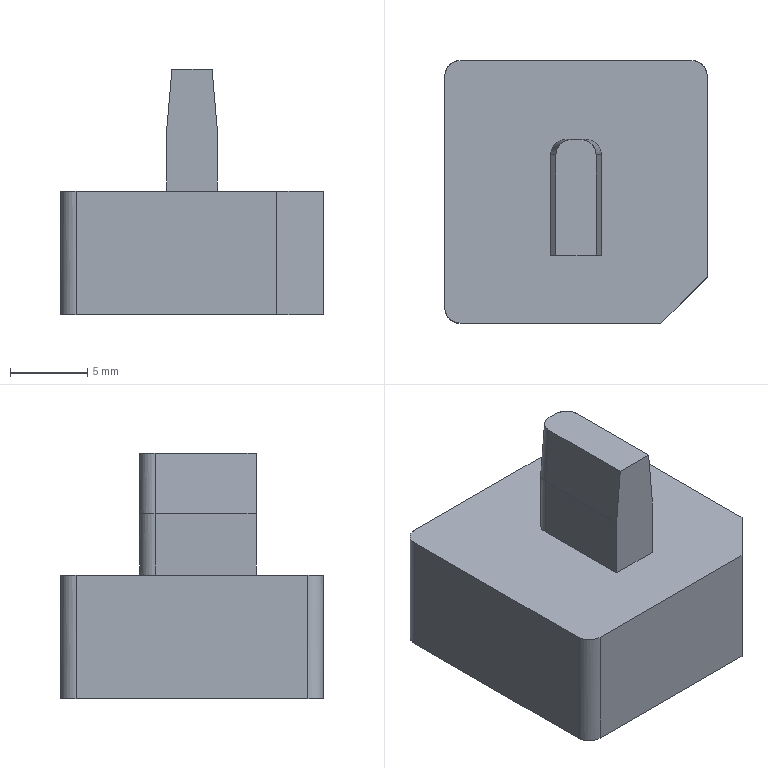NC program | PowerMill | posted with a generic post | part box 17 x 17 x 15.883 mm
Lines 1 to 1082 of 37483:
%
O0001
N104 ( POWERMILL CB  : 2026004.0)
N105 ( POST VER      : 2026.0.0.5161)
N106 ( OPTION FILE   : FANUC)
N107 ( OUTPUT WORKPLANE : WORLD)
N108 (  )
N109 ( TOOL LIST )
N110 (---------------------------------------)
N111 ( NO. | ID        | DIA.| TIP RAD|LENGTH)
N112 (---------------------------------------)
N113 (    1|D10C_1_1   |10.0 |  0.0   |71.32 )
N114 (    3|D10_1_1    |10.0 |  0.0   |71.04 )
N115 (   14|D4_1_1     | 4.0 |  0.0   |63.04 )
N116 (   13|TEXT_D4_1_1| 4.0 |  0.3   |63.16 )
N117 (---------------------------------------)
N118 (  )
N119 ( NUMBER OF TOOLPATHS: 9.0 )
N120 ( ESTIMATED PROGRAM DURATION: 0 HOURS 4 MIN 27 SEC)
N121 (  )
N122 G00 G21 G80 G40 G17
N123 G90
N124 G54
N125 G53 Z0.0
N126 (---------------)
N127 ( START TOOLPATH : 精公开粗01-扫面平行-D10C )
N128 (---------------)
N129 ( TOOL NO.    :1 )
N130 ( TOOL TYPE   : ENDMILL)
N131 ( TOOL ID     : D10C_1_1)
N132 ( TOOL DIA    : 10.0 LENGTH 71.32)
N133 T1
N134 M6
N135 S8000 M03
N136 G00 G90 X0.0 Y0.0
N137 G43 Z10.2 H1
N138
N139 G05 P10000 R4
N140 X11.28 Y11.28
N141 Z1.134
N142 G01 Z-0.066 F6000.0
N143 X-11.28 F10000.0
N144 Y5.64
N145 X11.28
N146 Y0.0
N147 X-11.28
N148 Y-5.64
N149 X11.28
N150 Y-11.28
N151 X-11.28
N152 X-16.28
N153 G00 Z10.2
N154 G05 P0
N155 (---------------)
N156 ( END TOOLPATH : 精公开粗01-扫面平行-D10C )
N157 (---------------)
N158 ( START TOOLPATH : 精公开粗01-外形偏置-D10C )
N159 (---------------)
N160 G00 X0.0 Y-0.3245 Z9.884
N161 G05 P10000 R4
N162 X6.2233 Y-17.204
N163 Z0.6953
N164 G01 Z-0.5047 F6000.0
N165 Y-16.6765 F10000.0
N166 G03 X1.4758 Y-11.929 I-4.7475 J0.0
N167 G01 X-10.28
N168 G02 X-11.28 Y-10.929 I0.0 J1.0
N169 G01 Y10.28
N170 G02 X-10.28 Y11.28 I1.0 J0.0
N171 G01 X10.28
N172 G02 X11.28 Y10.28 I0.0 J-1.0
N173 G01 Y-10.929
N174 G02 X10.28 Y-11.929 I-1.0 J0.0
N175 G01 X1.4758
N176 X1.3535 Y-9.4205
N177 X1.1601 Y-9.4299
N178 X-1.1601
N179 X-1.9336 Y-9.3922
N180 X-2.707 Y-9.2455
N181 X-3.4804 Y-8.9698
N182 X-3.7658 Y-8.8322
N183 X-4.2538 Y-8.5428
N184 X-4.8751 Y-8.0588
N185 X-5.0273 Y-7.9148
N186 X-5.5738 Y-7.2853
N187 X-5.8007 Y-6.9515
N188 X-6.0478 Y-6.5119
N189 X-6.3609 Y-5.7385
N190 X-6.5423 Y-4.9651
N191 X-6.6054 Y-4.1916
N192 X-6.6056 Y1.9958
N193 X-6.5917 Y2.7692
N194 X-6.4881 Y3.5426
N195 X-6.3018 Y4.3161
N196 X-5.9828 Y5.0895
N197 X-5.554 Y5.8629
N198 X-5.0273 Y6.5406
N199 X-4.2538 Y7.2833
N200 X-3.4804 Y7.8088
N201 X-2.7303 Y8.1832
N202 X-1.9336 Y8.455
N203 X-1.1601 Y8.6004
N204 X-0.3867 Y8.6667
N205 X0.3867
N206 X1.1601 Y8.6064
N207 X1.9336 Y8.4558
N208 X2.7363 Y8.1832
N209 X3.4804 Y7.8114
N210 X4.2538 Y7.285
N211 X4.9451 Y6.6363
N212 X5.5496 Y5.8629
N213 X5.8007 Y5.4567
N214 X5.994 Y5.0895
N215 X6.297 Y4.3161
N216 X6.4973 Y3.5426
N217 X6.5741 Y2.9617
N218 X6.6056 Y1.9958
N219 X6.6054 Y-4.1916
N220 X6.5423 Y-4.9651
N221 X6.3609 Y-5.7385
N222 X6.0478 Y-6.5119
N223 X5.8007 Y-6.9515
N224 X5.5738 Y-7.2853
N225 X5.0273 Y-7.9148
N226 X4.8751 Y-8.0588
N227 X4.2538 Y-8.5428
N228 X3.7658 Y-8.8322
N229 X3.4804 Y-8.9698
N230 X2.707 Y-9.2455
N231 X1.9336 Y-9.3922
N232 X1.3535 Y-9.4205
N233 X1.4758 Y-11.929
N234 G00 Z3.3066
N235 G01 X6.2233 Y-17.204
N236 G00 Z0.3066
N237 G01 Z-0.8934 F6000.0
N238 Y-16.6765 F10000.0
N239 G03 X1.4758 Y-11.929 I-4.7475 J0.0
N240 G01 X1.3581
N241 X1.2568 Y-9.426
N242 X1.1601 Y-9.4299
N243 X-1.1601
N244 X-1.9336 Y-9.3986
N245 X-2.707 Y-9.254
N246 X-3.4804 Y-8.9845
N247 X-3.7998 Y-8.8322
N248 X-4.2538 Y-8.5647
N249 X-4.9091 Y-8.0588
N250 X-5.6078 Y-7.2853
N251 X-5.8007 Y-7.0056
N252 X-6.0818 Y-6.5119
N253 X-6.395 Y-5.7385
N254 X-6.5741 Y-4.9786
N255 X-6.6394 Y-4.1916
N256 X-6.6396 Y1.9958
N257 X-6.6257 Y2.7692
N258 X-6.5221 Y3.5426
N259 X-6.3358 Y4.3161
N260 X-6.0168 Y5.0895
N261 X-5.588 Y5.8629
N262 X-5.0273 Y6.5771
N263 X-4.2538 Y7.3101
N264 X-3.4804 Y7.8271
N265 X-2.7643 Y8.1832
N266 X-1.9336 Y8.4632
N267 X-1.1601 Y8.6054
N268 X-0.3867 Y8.667
N269 X0.3867
N270 X1.1601 Y8.6109
N271 X1.9336 Y8.4645
N272 X2.707 Y8.208
N273 X3.4804 Y7.8315
N274 X4.1268 Y7.4098
N275 X4.9794 Y6.6363
N276 X5.5835 Y5.8629
N277 X6.028 Y5.0895
N278 X6.3309 Y4.3161
N279 X6.5314 Y3.5426
N280 X6.6257 Y2.7692
N281 X6.6396 Y1.9958
N282 X6.6394 Y-4.1916
N283 X6.5763 Y-4.9651
N284 X6.395 Y-5.7385
N285 X6.0818 Y-6.5119
N286 X5.8007 Y-7.0056
N287 X5.6078 Y-7.2853
N288 X5.0273 Y-7.947
N289 X4.2538 Y-8.5647
N290 X3.7998 Y-8.8322
N291 X3.4804 Y-8.9845
N292 X2.707 Y-9.254
N293 X1.9336 Y-9.3986
N294 X1.2568 Y-9.426
N295 X1.3581 Y-11.929
N296 X-10.28
N297 G02 X-11.28 Y-10.929 I0.0 J1.0
N298 G01 Y10.28
N299 G02 X-10.28 Y11.28 I1.0 J0.0
N300 G01 X10.28
N301 G02 X11.28 Y10.28 I0.0 J-1.0
N302 G01 Y-10.929
N303 G02 X10.28 Y-11.929 I-1.0 J0.0
N304 G01 X1.4758
N305 G00 Z2.9179
N306 G01 X6.2233 Y-17.204
N307 G00 Z-0.0821
N308 G01 Z-1.2821 F6000.0
N309 Y-16.6765 F10000.0
N310 G03 X1.4758 Y-11.929 I-4.7475 J0.0
N311 G01 X1.1601
N312 Y-9.4299
N313 X-1.1601
N314 X-1.9336 Y-9.4022
N315 X-2.707 Y-9.2626
N316 X-3.4804 Y-8.9992
N317 X-3.8338 Y-8.8322
N318 X-4.2538 Y-8.5867
N319 X-4.9431 Y-8.0588
N320 X-5.6418 Y-7.2853
N321 X-5.8007 Y-7.057
N322 X-6.1158 Y-6.5119
N323 X-6.429 Y-5.7385
N324 X-6.6103 Y-4.9651
N325 X-6.6734 Y-4.1916
N326 X-6.6736 Y1.9958
N327 X-6.6597 Y2.7692
N328 X-6.5741 Y3.4297
N329 X-6.3698 Y4.3161
N330 X-6.0508 Y5.0895
N331 X-5.622 Y5.8629
N332 X-5.0273 Y6.6135
N333 X-4.2538 Y7.3369
N334 X-3.4804 Y7.8453
N335 X-2.7983 Y8.1832
N336 X-1.9336 Y8.4715
N337 X-1.1601 Y8.6104
N338 X-0.3867 Y8.667
N339 X0.3867
N340 X1.1601 Y8.6153
N341 X1.9336 Y8.4729
N342 X2.707 Y8.2211
N343 X3.4804 Y7.8515
N344 X4.1607 Y7.4098
N345 X5.0138 Y6.6363
N346 X5.6174 Y5.8629
N347 X6.062 Y5.0895
N348 X6.3648 Y4.3161
N349 X6.5654 Y3.5426
N350 X6.6597 Y2.7692
N351 X6.6735 Y1.9958
N352 X6.6734 Y-4.1916
N353 X6.6103 Y-4.9651
N354 X6.429 Y-5.7385
N355 X6.1158 Y-6.5119
N356 X5.8007 Y-7.057
N357 X5.6418 Y-7.2853
N358 X5.0273 Y-7.9791
N359 X4.2538 Y-8.5867
N360 X3.8338 Y-8.8322
N361 X3.4804 Y-8.9992
N362 X2.707 Y-9.2626
N363 X1.9336 Y-9.4022
N364 X1.1601 Y-9.4299
N365 Y-11.929
N366 X-10.28
N367 G02 X-11.28 Y-10.929 I0.0 J1.0
N368 G01 Y10.28
N369 G02 X-10.28 Y11.28 I1.0 J0.0
N370 G01 X10.28
N371 G02 X11.28 Y10.28 I0.0 J-1.0
N372 G01 Y-10.929
N373 G02 X10.28 Y-11.929 I-1.0 J0.0
N374 G01 X1.4758
N375 G00 Z2.5292
N376 G01 X6.2233 Y-17.204
N377 G00 Z-0.4708
N378 G01 Z-1.6708 F6000.0
N379 Y-16.6765 F10000.0
N380 G03 X1.4758 Y-11.929 I-4.7475 J0.0
N381 G01 X1.1601
N382 Y-9.4299
N383 X-1.1601
N384 X-1.9336 Y-9.4056
N385 X-2.707 Y-9.2711
N386 X-3.4804 Y-9.0138
N387 X-3.8678 Y-8.8322
N388 X-4.2538 Y-8.6086
N389 X-4.9771 Y-8.0588
N390 X-5.6758 Y-7.2853
N391 X-6.1497 Y-6.5119
N392 X-6.463 Y-5.7385
N393 X-6.6443 Y-4.9651
N394 X-6.7074 Y-4.1916
N395 X-6.7076 Y1.9958
N396 X-6.6937 Y2.7692
N397 X-6.5902 Y3.5426
N398 X-6.4038 Y4.3161
N399 X-6.0848 Y5.0895
N400 X-5.656 Y5.8629
N401 X-5.04 Y6.6363
N402 X-4.2538 Y7.3637
N403 X-3.4804 Y7.8636
N404 X-2.8323 Y8.1832
N405 X-1.9336 Y8.4798
N406 X-1.1601 Y8.6154
N407 X-0.3867 Y8.667
N408 X0.3867
N409 X1.1601 Y8.6197
N410 X1.9336 Y8.4814
N411 X2.707 Y8.2343
N412 X3.4804 Y7.8715
N413 X4.1947 Y7.4098
N414 X5.048 Y6.6363
N415 X5.6513 Y5.8629
N416 X6.096 Y5.0895
N417 X6.3987 Y4.3161
N418 X6.5741 Y3.6729
N419 X6.6938 Y2.7692
N420 X6.7075 Y1.9958
N421 X6.7074 Y-4.1916
N422 X6.6443 Y-4.9651
N423 X6.463 Y-5.7385
N424 X6.1497 Y-6.5119
N425 X5.6758 Y-7.2853
N426 X5.0273 Y-8.0113
N427 X4.2538 Y-8.6086
N428 X3.8678 Y-8.8322
N429 X3.4804 Y-9.0138
N430 X2.707 Y-9.2711
N431 X1.9336 Y-9.4056
N432 X1.1601 Y-9.4299
N433 Y-11.929
N434 X-10.28
N435 G02 X-11.28 Y-10.929 I0.0 J1.0
N436 G01 Y10.28
N437 G02 X-10.28 Y11.28 I1.0 J0.0
N438 G01 X10.28
N439 G02 X11.28 Y10.28 I0.0 J-1.0
N440 G01 Y-10.929
N441 G02 X10.28 Y-11.929 I-1.0 J0.0
N442 G01 X1.4758
N443 G00 Z2.1405
N444 G01 X6.2233 Y-17.204
N445 G00 Z-0.8595
N446 G01 Z-2.0595 F6000.0
N447 Y-16.6765 F10000.0
N448 G03 X1.4758 Y-11.929 I-4.7475 J0.0
N449 G01 X-10.28
N450 G02 X-11.28 Y-10.929 I0.0 J1.0
N451 G01 Y10.28
N452 G02 X-10.28 Y11.28 I1.0 J0.0
N453 G01 X10.28
N454 G02 X11.28 Y10.28 I0.0 J-1.0
N455 G01 Y-10.929
N456 G02 X10.28 Y-11.929 I-1.0 J0.0
N457 G01 X2.0024
N458 X1.9336 Y-9.4088
N459 X1.1601 Y-9.4299
N460 X-1.1601
N461 X-1.9336 Y-9.4088
N462 X-2.707 Y-9.2796
N463 X-3.4804 Y-9.0285
N464 X-3.9018 Y-8.8322
N465 X-4.2538 Y-8.6306
N466 X-5.0111 Y-8.0588
N467 X-5.7098 Y-7.2853
N468 X-6.1837 Y-6.5119
N469 X-6.497 Y-5.7385
N470 X-6.6783 Y-4.9651
N471 X-6.7413 Y-4.1916
N472 X-6.7416 Y1.9958
N473 X-6.7277 Y2.7692
N474 X-6.6242 Y3.5426
N475 X-6.4378 Y4.3161
N476 X-6.1188 Y5.0895
N477 X-5.69 Y5.8629
N478 X-5.074 Y6.6363
N479 X-4.2294 Y7.4098
N480 X-3.4804 Y7.8819
N481 X-2.8663 Y8.1832
N482 X-1.9336 Y8.4878
N483 X-1.1601 Y8.6201
N484 X-0.3867 Y8.667
N485 X0.3867
N486 X1.1601 Y8.624
N487 X1.9336 Y8.4899
N488 X2.707 Y8.2474
N489 X3.4804 Y7.8914
N490 X4.2286 Y7.4098
N491 X5.0273 Y6.694
N492 X5.6852 Y5.8629
N493 X6.13 Y5.0895
N494 X6.4326 Y4.3161
N495 X6.6336 Y3.5426
N496 X6.7278 Y2.7692
N497 X6.7415 Y1.9958
N498 X6.7414 Y-4.1916
N499 X6.6783 Y-4.9651
N500 X6.497 Y-5.7385
N501 X6.1837 Y-6.5119
N502 X5.7098 Y-7.2853
N503 X5.0111 Y-8.0588
N504 X4.2538 Y-8.6306
N505 X3.9018 Y-8.8322
N506 X3.4804 Y-9.0285
N507 X2.707 Y-9.2796
N508 X1.9336 Y-9.4088
N509 X2.0024 Y-11.929
N510 X1.4758
N511 G00 Z1.7518
N512 G01 X6.2233 Y-17.204
N513 G00 Z-1.2482
N514 G01 Z-2.4482 F6000.0
N515 Y-16.6765 F10000.0
N516 G03 X1.4758 Y-11.929 I-4.7475 J0.0
N517 G01 X-10.28
N518 G02 X-11.28 Y-10.929 I0.0 J1.0
N519 G01 Y10.28
N520 G02 X-10.28 Y11.28 I1.0 J0.0
N521 G01 X10.28
N522 G02 X11.28 Y10.28 I0.0 J-1.0
N523 G01 Y-10.929
N524 G02 X10.28 Y-11.929 I-1.0 J0.0
N525 G01 X1.9931
N526 X1.9336 Y-9.4117
N527 X1.1601 Y-9.4299
N528 X1.1509
N529 X-1.1601
N530 X-1.7978 Y-9.4125
N531 X-1.9336 Y-9.4117
N532 X-2.707 Y-9.2881
N533 X-3.4804 Y-9.0423
N534 X-3.9358 Y-8.8322
N535 X-4.2538 Y-8.652
N536 X-5.0451 Y-8.0588
N537 X-5.7439 Y-7.2853
N538 X-6.2177 Y-6.5119
N539 X-6.531 Y-5.7385
N540 X-6.7123 Y-4.9651
N541 X-6.7753 Y-4.1916
N542 X-6.7756 Y1.9958
N543 X-6.7617 Y2.7692
N544 X-6.6582 Y3.5426
N545 X-6.4718 Y4.3161
N546 X-6.1528 Y5.0895
N547 X-5.8007 Y5.7413
N548 X-5.108 Y6.6363
N549 X-4.2634 Y7.4098
N550 X-3.4804 Y7.8997
N551 X-2.707 Y8.2616
N552 X-1.9336 Y8.4954
N553 X-1.1601 Y8.6245
N554 X-0.3867 Y8.667
N555 X0.3867
N556 X1.1601 Y8.6282
N557 X1.9336 Y8.4983
N558 X2.707 Y8.2605
N559 X3.4804 Y7.9096
N560 X4.2538 Y7.4162
N561 X5.0273 Y6.7299
N562 X5.7191 Y5.8629
N563 X6.164 Y5.0895
N564 X6.4665 Y4.3161
N565 X6.5741 Y3.9618
N566 X6.6677 Y3.5426
N567 X6.7618 Y2.7692
N568 X6.7755 Y1.9958
N569 X6.7754 Y-4.1916
N570 X6.7123 Y-4.9651
N571 X6.5741 Y-5.5936
N572 X6.2177 Y-6.5119
N573 X5.8007 Y-7.2051
N574 X5.0451 Y-8.0588
N575 X4.2538 Y-8.652
N576 X3.9358 Y-8.8322
N577 X3.4804 Y-9.0423
N578 X2.707 Y-9.2881
N579 X1.9336 Y-9.4117
N580 X1.9931 Y-11.929
N581 X1.4758
N582 G00 Z1.3631
N583 G01 X6.2233 Y-17.204
N584 G00 Z-1.6369
N585 G01 Z-2.8369 F6000.0
N586 Y-16.6765 F10000.0
N587 G03 X1.4758 Y-11.929 I-4.7475 J0.0
N588 G01 X-10.28
N589 G02 X-11.28 Y-10.929 I0.0 J1.0
N590 G01 Y10.28
N591 G02 X-10.28 Y11.28 I1.0 J0.0
N592 G01 X10.28
N593 G02 X11.28 Y10.28 I0.0 J-1.0
N594 G01 Y-10.929
N595 G02 X10.28 Y-11.929 I-1.0 J0.0
N596 G01 X1.984
N597 X1.9336 Y-9.4144
N598 X1.1601 Y-9.4299
N599 X1.1383 Y-9.4298
N600 X-1.1601
N601 X-1.677 Y-9.4157
N602 X-1.9336 Y-9.4144
N603 X-2.707 Y-9.2966
N604 X-3.4804 Y-9.0556
N605 X-3.9698 Y-8.8322
N606 X-4.2538 Y-8.6721
N607 X-5.0273 Y-8.104
N608 X-5.7779 Y-7.2853
N609 X-6.2517 Y-6.5119
N610 X-6.565 Y-5.7385
N611 X-6.7463 Y-4.9651
N612 X-6.8093 Y-4.1916
N613 X-6.8096 Y1.9958
N614 X-6.7957 Y2.7692
N615 X-6.6922 Y3.5426
N616 X-6.5058 Y4.3161
N617 X-6.1868 Y5.0895
N618 X-5.8007 Y5.796
N619 X-5.142 Y6.6363
N620 X-4.2974 Y7.4098
N621 X-3.4804 Y7.9171
N622 X-2.707 Y8.2754
N623 X-1.9336 Y8.5027
N624 X-1.1601 Y8.6288
N625 X-0.3867 Y8.667
N626 X0.3867
N627 X1.1601 Y8.6323
N628 X1.9336 Y8.5068
N629 X2.707 Y8.2736
N630 X3.4804 Y7.9278
N631 X4.2538 Y7.441
N632 X5.1506 Y6.6363
N633 X5.753 Y5.8629
N634 X6.198 Y5.0895
N635 X6.5003 Y4.3161
N636 X6.7018 Y3.5426
N637 X6.7958 Y2.7692
N638 X6.8095 Y1.9958
N639 X6.8094 Y-4.1916
N640 X6.7463 Y-4.9651
N641 X6.565 Y-5.7385
N642 X6.2517 Y-6.5119
N643 X5.8007 Y-7.2531
N644 X5.0791 Y-8.0588
N645 X4.2538 Y-8.6721
N646 X3.9698 Y-8.8322
N647 X3.4804 Y-9.0556
N648 X2.707 Y-9.2966
N649 X1.9336 Y-9.4144
N650 X1.984 Y-11.929
N651 X1.4758
N652 G00 Z0.9744
N653 G01 X6.2233 Y-17.204
N654 G00 Z-2.0256
N655 G01 Z-3.2256 F6000.0
N656 Y-16.6765 F10000.0
N657 G03 X1.4758 Y-11.929 I-4.7475 J0.0
N658 G01 X-10.28
N659 G02 X-11.28 Y-10.929 I0.0 J1.0
N660 G01 Y10.28
N661 G02 X-10.28 Y11.28 I1.0 J0.0
N662 G01 X10.28
N663 G02 X11.28 Y10.28 I0.0 J-1.0
N664 G01 Y-10.929
N665 G02 X10.28 Y-11.929 I-1.0 J0.0
N666 G01 X1.9336
N667 Y-9.417
N668 X1.8047
N669 X1.1601 Y-9.4299
N670 X1.1383 Y-9.4298
N671 X-1.1601
N672 X-1.6295 Y-9.417
N673 X-1.9336
N674 X-2.707 Y-9.3046
N675 X-3.4804 Y-9.0689
N676 X-4.0038 Y-8.8322
N677 X-4.2538 Y-8.6923
N678 X-5.0273 Y-8.1336
N679 X-5.8007 Y-7.3
N680 X-6.2857 Y-6.5119
N681 X-6.5741 Y-5.8139
N682 X-6.7803 Y-4.9651
N683 X-6.8433 Y-4.1916
N684 X-6.8436 Y1.9958
N685 X-6.8297 Y2.7692
N686 X-6.7262 Y3.5426
N687 X-6.5741 Y4.2046
N688 X-6.2209 Y5.0895
N689 X-5.8007 Y5.8493
N690 X-5.176 Y6.6363
N691 X-4.3314 Y7.4098
N692 X-3.4804 Y7.9346
N693 X-2.707 Y8.2879
N694 X-1.9336 Y8.5098
N695 X-1.1601 Y8.6328
N696 X-0.3867 Y8.667
N697 X0.3867
N698 X1.1601 Y8.6364
N699 X1.9336 Y8.5146
N700 X2.707 Y8.2867
N701 X3.4804 Y7.946
N702 X4.2538 Y7.4659
N703 X5.0273 Y6.8016
N704 X5.1848 Y6.6363
N705 X5.7868 Y5.8629
N706 X6.232 Y5.0895
N707 X6.5342 Y4.3161
N708 X6.7359 Y3.5426
N709 X6.8298 Y2.7692
N710 X6.8435 Y1.9958
N711 X6.8434 Y-4.1916
N712 X6.7803 Y-4.9651
N713 X6.599 Y-5.7385
N714 X6.2857 Y-6.5119
N715 X5.8119 Y-7.2853
N716 X5.1131 Y-8.0588
N717 X4.2538 Y-8.6923
N718 X4.0038 Y-8.8322
N719 X3.4804 Y-9.0689
N720 X2.707 Y-9.3046
N721 X1.9336 Y-9.417
N722 Y-11.929
N723 X1.4758
N724 G00 Z0.5857
N725 G01 X6.2233 Y-17.204
N726 G00 Z-2.4143
N727 G01 Z-3.6143 F6000.0
N728 Y-16.6765 F10000.0
N729 G03 X1.4758 Y-11.929 I-4.7475 J0.0
N730 G01 X-10.28
N731 G02 X-11.28 Y-10.929 I0.0 J1.0
N732 G01 Y10.28
N733 G02 X-10.28 Y11.28 I1.0 J0.0
N734 G01 X10.28
N735 G02 X11.28 Y10.28 I0.0 J-1.0
N736 G01 Y-10.929
N737 G02 X10.28 Y-11.929 I-1.0 J0.0
N738 G01 X1.9336
N739 Y-9.4192
N740 X1.6884
N741 X1.1601 Y-9.4298
N742 X1.1383 Y-9.4297
N743 X-1.1601
N744 X-1.5441 Y-9.4192
N745 X-1.9336
N746 X-2.707 Y-9.3121
N747 X-3.4804 Y-9.0822
N748 X-3.9979 Y-8.8348
N749 X-4.0038 Y-8.8321
N750 X-4.0057 Y-8.8311
N751 X-4.2538 Y-8.7124
N752 X-5.1471 Y-8.0588
N753 X-5.8007 Y-7.3448
N754 X-6.3197 Y-6.5119
N755 X-6.5741 Y-5.914
N756 X-6.8143 Y-4.9651
N757 X-6.8773 Y-4.1916
N758 X-6.8776 Y1.9958
N759 X-6.8637 Y2.7692
N760 X-6.7602 Y3.5426
N761 X-6.5741 Y4.3151
N762 X-6.2549 Y5.0895
N763 X-5.8265 Y5.8629
N764 X-5.2101 Y6.6363
N765 X-4.3654 Y7.4098
N766 X-3.4804 Y7.952
N767 X-2.707 Y8.3004
N768 X-1.9336 Y8.5167
N769 X-1.1601 Y8.6365
N770 X-0.3867 Y8.6671
N771 X-0.3835 Y8.667
N772 X0.3867
N773 X0.9799 Y8.6435
N774 X1.1601 Y8.6404
N775 X1.9336 Y8.5222
N776 X2.707 Y8.2999
N777 X3.4804 Y7.9642
N778 X4.2538 Y7.4908
N779 X5.0273 Y6.8361
N780 X5.219 Y6.6363
N781 X5.8007 Y5.8936
N782 X6.266 Y5.0895
N783 X6.5681 Y4.3161
N784 X6.7699 Y3.5426
N785 X6.8638 Y2.7692
N786 X6.8775 Y1.9958
N787 X6.8774 Y-4.1916
N788 X6.8143 Y-4.9651
N789 X6.6329 Y-5.7385
N790 X6.3197 Y-6.5119
N791 X5.8458 Y-7.2853
N792 X5.1471 Y-8.0588
N793 X4.2538 Y-8.7124
N794 X4.0378 Y-8.8322
N795 X3.4804 Y-9.0822
N796 X2.707 Y-9.3121
N797 X1.9336 Y-9.4192
N798 Y-11.929
N799 X1.4758
N800 G00 Z0.197
N801 G01 X6.2233 Y-17.204
N802 G00 Z-2.803
N803 G01 Z-4.003 F6000.0
N804 Y-16.6765 F10000.0
N805 G03 X1.4758 Y-11.929 I-4.7475 J0.0
N806 G01 X-10.28
N807 G02 X-11.28 Y-10.929 I0.0 J1.0
N808 G01 Y10.28
N809 G02 X-10.28 Y11.28 I1.0 J0.0
N810 G01 X10.28
N811 G02 X11.28 Y10.28 I0.0 J-1.0
N812 G01 Y-10.929
N813 G02 X10.28 Y-11.929 I-1.0 J0.0
N814 G01 X1.9336
N815 Y-9.4213
N816 X1.5821
N817 X1.1601 Y-9.4298
N818 X1.1383 Y-9.4297
N819 X-1.1601
N820 X-1.466 Y-9.4213
N821 X-1.9336
N822 X-2.707 Y-9.3193
N823 X-3.4804 Y-9.0955
N824 X-4.2538 Y-8.7326
N825 X-5.0273 Y-8.1929
N826 X-5.1811 Y-8.0588
N827 X-5.8007 Y-7.3896
N828 X-6.3537 Y-6.5119
N829 X-6.6669 Y-5.7385
N830 X-6.8483 Y-4.9651
N831 X-6.9113 Y-4.1916
N832 X-6.9116 Y1.9958
N833 X-6.8977 Y2.7692
N834 X-6.7942 Y3.5426
N835 X-6.6078 Y4.3161
N836 X-6.2889 Y5.0895
N837 X-5.8611 Y5.8629
N838 X-5.2441 Y6.6363
N839 X-5.0273 Y6.8593
N840 X-4.3993 Y7.4098
N841 X-3.4804 Y7.9694
N842 X-3.0364 Y8.1832
N843 X-2.707 Y8.3128
N844 X-1.9336 Y8.5234
N845 X-1.1601 Y8.6401
N846 X-0.3867 Y8.6671
N847 X-0.3792 Y8.6669
N848 X0.3867
N849 X0.8394 Y8.649
N850 X1.1601 Y8.6443
N851 X1.9336 Y8.5297
N852 X2.707 Y8.313
N853 X3.4804 Y7.9824
N854 X4.2538 Y7.5157
N855 X5.0273 Y6.8707
N856 X5.2532 Y6.6363
N857 X5.8007 Y5.9454
N858 X6.3 Y5.0895
N859 X6.5741 Y4.3984
N860 X6.804 Y3.5426
N861 X6.8978 Y2.7692
N862 X6.9114 Y1.9958
N863 Y-4.1916
N864 X6.8483 Y-4.9651
N865 X6.6669 Y-5.7385
N866 X6.3537 Y-6.5119
N867 X5.8798 Y-7.2853
N868 X5.1811 Y-8.0588
N869 X5.0273 Y-8.1929
N870 X4.2538 Y-8.7326
N871 X4.0718 Y-8.8322
N872 X3.4804 Y-9.0955
N873 X2.707 Y-9.3193
N874 X1.9336 Y-9.4213
N875 Y-11.929
N876 X1.4758
N877 G00 Z-0.1917
N878 G01 X6.2233 Y-17.204
N879 G00 Z-3.1917
N880 G01 Z-4.3917 F6000.0
N881 Y-16.6765 F10000.0
N882 G03 X1.4758 Y-11.929 I-4.7475 J0.0
N883 G01 X-10.28
N884 G02 X-11.28 Y-10.929 I0.0 J1.0
N885 G01 Y10.28
N886 G02 X-10.28 Y11.28 I1.0 J0.0
N887 G01 X10.28
N888 G02 X11.28 Y10.28 I0.0 J-1.0
N889 G01 Y-10.929
N890 G02 X10.28 Y-11.929 I-1.0 J0.0
N891 G01 X1.9336
N892 Y-9.4218
N893 X1.557
N894 X1.1601 Y-9.4297
N895 X1.1383 Y-9.4296
N896 X-1.1601
N897 X-1.4476 Y-9.4218
N898 X-1.9336
N899 X-2.707 Y-9.3208
N900 X-3.4804 Y-9.0985
N901 X-4.2538 Y-8.737
N902 X-5.0273 Y-8.1995
N903 X-5.1887 Y-8.0588
N904 X-5.8007 Y-7.3994
N905 X-6.3613 Y-6.5119
N906 X-6.5741 Y-6.027
N907 X-6.6744 Y-5.7385
N908 X-6.8557 Y-4.9651
N909 X-6.9189 Y-4.1916
N910 X-6.919 Y1.9958
N911 X-6.9052 Y2.7692
N912 X-6.8116 Y3.5426
N913 X-6.6152 Y4.3161
N914 X-6.3059 Y5.0895
N915 X-5.8687 Y5.8629
N916 X-5.2606 Y6.6363
N917 X-5.0273 Y6.8783
N918 X-4.4069 Y7.4098
N919 X-3.4804 Y7.9826
N920 X-3.054 Y8.1832
N921 X-2.707 Y8.3156
N922 X-1.9336 Y8.5314
N923 X-1.1601 Y8.6409
N924 X-0.3867 Y8.6671
N925 X-0.375 Y8.6669
N926 X0.3867
N927 X0.8123 Y8.65
N928 X1.1601 Y8.6451
N929 X1.9336 Y8.5314
N930 X2.707 Y8.3159
N931 X3.4804 Y7.9864
N932 X4.2538 Y7.5211
N933 X5.0273 Y6.8783
N934 X5.2607 Y6.6363
N935 X5.8007 Y5.9627
N936 X6.3074 Y5.0895
N937 X6.5741 Y4.4351
N938 X6.8117 Y3.5426
N939 X6.9069 Y2.7692
N940 X6.9191 Y1.9958
N941 X6.9189 Y-4.1916
N942 X6.8557 Y-4.9651
N943 X6.6744 Y-5.7385
N944 X6.5741 Y-6.027
N945 X6.3613 Y-6.5119
N946 X5.8873 Y-7.2853
N947 X5.1887 Y-8.0588
N948 X5.0273 Y-8.1995
N949 X4.2538 Y-8.737
N950 X4.0794 Y-8.8322
N951 X3.4804 Y-9.0985
N952 X2.707 Y-9.3208
N953 X1.9336 Y-9.4218
N954 Y-11.929
N955 X1.4758
N956 G00 Z-0.5804
N957 G01 X6.2233 Y-17.204
N958 G00 Z-3.5804
N959 G01 Z-4.7804 F6000.0
N960 Y-16.6765 F10000.0
N961 G03 X1.4758 Y-11.929 I-4.7475 J0.0
N962 G01 X-10.28
N963 G02 X-11.28 Y-10.929 I0.0 J1.0
N964 G01 Y10.28
N965 G02 X-10.28 Y11.28 I1.0 J0.0
N966 G01 X10.28
N967 G02 X11.28 Y10.28 I0.0 J-1.0
N968 G01 Y-10.929
N969 G02 X10.28 Y-11.929 I-1.0 J0.0
N970 G01 X1.9336
N971 Y-9.4218
N972 X1.5541
N973 X1.1601 Y-9.4297
N974 X1.1383 Y-9.4296
N975 X-1.1601
N976 X-1.4454 Y-9.4218
N977 X-1.9336
N978 X-2.707 Y-9.3208
N979 X-3.4804 Y-9.0985
N980 X-4.2538 Y-8.737
N981 X-5.0273 Y-8.1995
N982 X-5.1887 Y-8.0588
N983 X-5.8007 Y-7.3994
N984 X-6.3613 Y-6.5119
N985 X-6.5741 Y-6.027
N986 X-6.6744 Y-5.7385
N987 X-6.8557 Y-4.9651
N988 X-6.9189 Y-4.1916
N989 X-6.919 Y1.9958
N990 X-6.9052 Y2.7692
N991 X-6.8116 Y3.5426
N992 X-6.6152 Y4.3161
N993 X-6.3061 Y5.0895
N994 X-5.8687 Y5.8629
N995 X-5.2606 Y6.6363
N996 X-5.0273 Y6.8783
N997 X-4.407 Y7.4098
N998 X-3.4804 Y7.983
N999 X-3.054 Y8.1832
N1000 X-2.707 Y8.3156
N1001 X-1.9336 Y8.5314
N1002 X-1.1601 Y8.6409
N1003 X-0.3867 Y8.6671
N1004 X-0.3712 Y8.6668
N1005 X0.3867
N1006 X0.81 Y8.6501
N1007 X1.1601 Y8.6451
N1008 X1.9336 Y8.5314
N1009 X2.707 Y8.3159
N1010 X3.4804 Y7.9864
N1011 X4.2538 Y7.5211
N1012 X5.0273 Y6.8783
N1013 X5.2607 Y6.6363
N1014 X5.8007 Y5.9627
N1015 X6.3074 Y5.0895
N1016 X6.5741 Y4.4351
N1017 X6.8117 Y3.5426
N1018 X6.907 Y2.7692
N1019 X6.9191 Y1.9958
N1020 X6.9189 Y-4.1916
N1021 X6.8557 Y-4.9651
N1022 X6.6744 Y-5.7385
N1023 X6.5741 Y-6.027
N1024 X6.3613 Y-6.5119
N1025 X5.8873 Y-7.2853
N1026 X5.1887 Y-8.0588
N1027 X5.0273 Y-8.1995
N1028 X4.2538 Y-8.737
N1029 X4.0794 Y-8.8322
N1030 X3.4804 Y-9.0985
N1031 X2.707 Y-9.3208
N1032 X1.9336 Y-9.4218
N1033 Y-11.929
N1034 X1.4758
N1035 G00 Z-0.9691
N1036 G01 X6.2233 Y-17.204
N1037 G00 Z-3.9691
N1038 G01 Z-5.1691 F6000.0
N1039 Y-16.6765 F10000.0
N1040 G03 X1.4758 Y-11.929 I-4.7475 J0.0
N1041 G01 X-10.28
N1042 G02 X-11.28 Y-10.929 I0.0 J1.0
N1043 G01 Y10.28
N1044 G02 X-10.28 Y11.28 I1.0 J0.0
N1045 G01 X10.28
N1046 G02 X11.28 Y10.28 I0.0 J-1.0
N1047 G01 Y-10.929
N1048 G02 X10.28 Y-11.929 I-1.0 J0.0
N1049 G01 X1.9336
N1050 Y-9.4218
N1051 X1.5511
N1052 X1.1601 Y-9.4296
N1053 X1.1383 Y-9.4295
N1054 X-1.1601
N1055 X-1.4432 Y-9.4218
N1056 X-1.9336
N1057 X-2.707 Y-9.3208
N1058 X-3.4804 Y-9.0985
N1059 X-4.2538 Y-8.737
N1060 X-5.0273 Y-8.1995
N1061 X-5.1887 Y-8.0588
N1062 X-5.8007 Y-7.3994
N1063 X-6.3614 Y-6.5119
N1064 X-6.5741 Y-6.027
N1065 X-6.6744 Y-5.7385
N1066 X-6.8557 Y-4.9651
N1067 X-6.9189 Y-4.1916
N1068 X-6.919 Y1.9958
N1069 X-6.9053 Y2.7692
N1070 X-6.8116 Y3.5426
N1071 X-6.6152 Y4.3161
N1072 X-6.3063 Y5.0895
N1073 X-5.8687 Y5.8629
N1074 X-5.2606 Y6.6363
N1075 X-5.0273 Y6.8783
N1076 X-4.407 Y7.4098
N1077 X-3.4804 Y7.9834
N1078 X-3.054 Y8.1832
N1079 X-2.707 Y8.3156
N1080 X-1.9336 Y8.5314
N1081 X-1.1601 Y8.6409
N1082 X-0.3867 Y8.6671
N1083 X-0.3672 Y8.6668
N1084 X0.3867
N1085 X0.8077 Y8.6501
N1086 X1.1601 Y8.6451
N1087 X1.9336 Y8.5314
N1088 X2.707 Y8.3159
N1089 X3.4804 Y7.9864
N1090 X4.2538 Y7.5211
N1091 X5.0273 Y6.8783
N1092 X5.2607 Y6.6363
N1093 X5.8007 Y5.9627
N1094 X6.3074 Y5.0895
N1095 X6.5741 Y4.4352
N1096 X6.8117 Y3.5426
N1097 X6.907 Y2.7692
N1098 X6.9191 Y1.9958
N1099 X6.9189 Y-4.1916
N1100 X6.8557 Y-4.9651
N1101 X6.6744 Y-5.7385
N1102 X6.5741 Y-6.027
N1103 X6.3614 Y-6.5119
N1104 X5.8873 Y-7.2853
N1105 X5.1887 Y-8.0588
N1106 X5.0273 Y-8.1995
N1107 X4.2538 Y-8.737
N1108 X4.0794 Y-8.8322
N1109 X3.4804 Y-9.0985
N1110 X2.707 Y-9.3208
N1111 X1.9336 Y-9.4218
N1112 Y-11.929
N1113 X1.4758
N1114 G00 Z-1.3578
N1115 G01 X6.2233 Y-17.204
N1116 G00 Z-4.3578
N1117 G01 Z-5.5578 F6000.0
N1118 Y-16.6765 F10000.0
N1119 G03 X1.4758 Y-11.929 I-4.7475 J0.0
N1120 G01 X-10.28
N1121 G02 X-11.28 Y-10.929 I0.0 J1.0
N1122 G01 Y10.28
N1123 G02 X-10.28 Y11.28 I1.0 J0.0
N1124 G01 X10.28
N1125 G02 X11.28 Y10.28 I0.0 J-1.0
N1126 G01 Y-10.929
N1127 G02 X10.28 Y-11.929 I-1.0 J0.0
N1128 G01 X1.9336
N1129 Y-9.4218
N1130 X1.5481
N1131 X1.1601 Y-9.4296
N1132 X1.1383 Y-9.4295
N1133 X-1.1601
N1134 X-1.4411 Y-9.4218
N1135 X-1.9336
N1136 X-2.707 Y-9.3208
N1137 X-3.4804 Y-9.0985
N1138 X-4.2538 Y-8.737
N1139 X-5.0273 Y-8.1995
N1140 X-5.1887 Y-8.0588
N1141 X-5.8007 Y-7.3995
N1142 X-6.3614 Y-6.5119
N1143 X-6.5741 Y-6.0271
N1144 X-6.6745 Y-5.7385
N1145 X-6.8557 Y-4.9651
N1146 X-6.9189 Y-4.1916
N1147 X-6.919 Y1.9958
N1148 X-6.9053 Y2.7692
N1149 X-6.8116 Y3.5426
N1150 X-6.6152 Y4.3161
N1151 X-6.3064 Y5.0895
N1152 X-5.8687 Y5.8629
N1153 X-5.2606 Y6.6363
N1154 X-5.0273 Y6.8783
N1155 X-4.407 Y7.4098
N1156 X-3.4804 Y7.9837
N1157 X-3.054 Y8.1832
N1158 X-2.707 Y8.3157
N1159 X-1.9336 Y8.5314
N1160 X-1.1601 Y8.6409
N1161 X-0.3867 Y8.6671
N1162 X-0.3634 Y8.6667
N1163 X0.3867
N1164 X0.8054 Y8.6501
N1165 X1.1601 Y8.6451
N1166 X1.9336 Y8.5314
N1167 X2.707 Y8.3159
N1168 X3.4804 Y7.9864
N1169 X4.2538 Y7.5211
N1170 X5.0273 Y6.8783
N1171 X5.2607 Y6.6363
N1172 X5.8007 Y5.9628
N1173 X6.3075 Y5.0895
N1174 X6.5741 Y4.4352
N1175 X6.8117 Y3.5426
N1176 X6.907 Y2.7692
N1177 X6.9191 Y1.9958
N1178 X6.9189 Y-4.1916
N1179 X6.8557 Y-4.9651